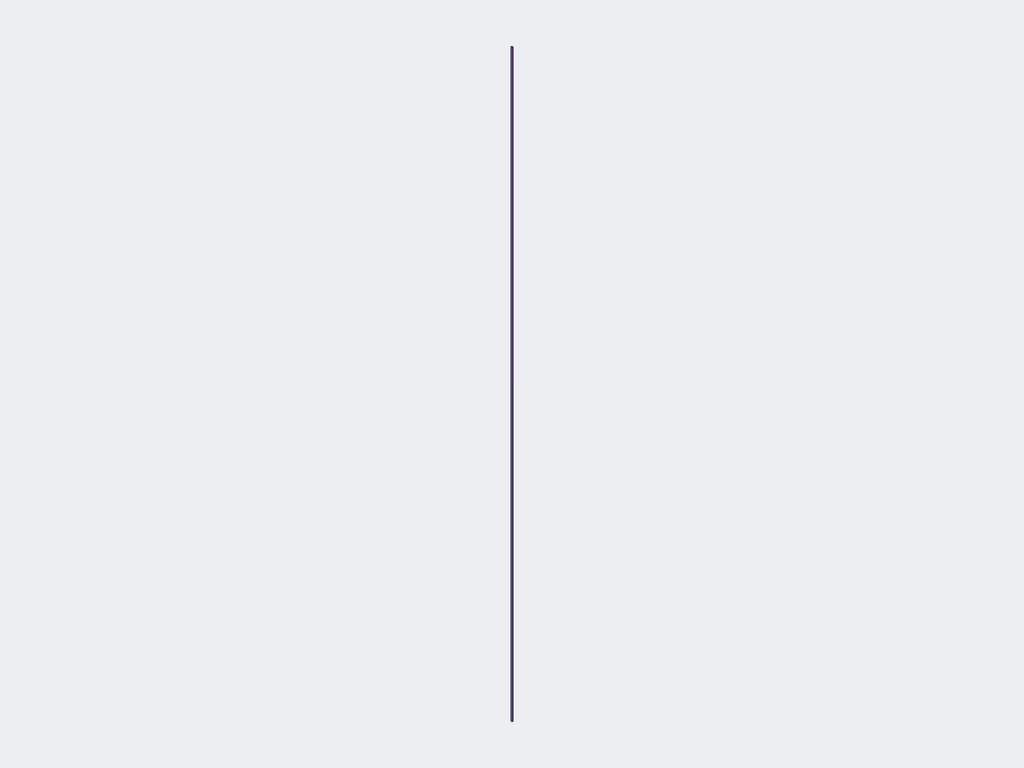Assembly | SolidWorks | 7 different items | 13 placed | box 6 x 6 x 1900 mm
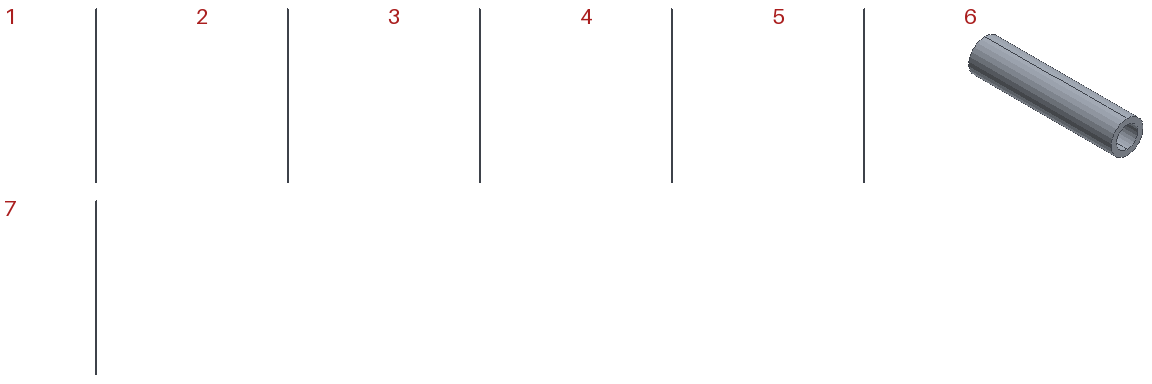Parts list (item | name | quantity | parent item | size | volume | features):
1 | (subassembly) | x1 | - | 3 x 3 x 1900 mm | 13430 mm3 | features CompositeCurve 18, Attribute 11
2 | - | x3 | in 1 | 0.15 x 0.15 x 1900 mm | 10.259 mm3 | features Extrusion 1
3 | - | x3 | in 1 | 0.3 x 0.3 x 1900 mm | 100.727 mm3 | features Extrusion 1
4 | - | x3 | in 1 | 0.125 x 0.125 x 1900 mm | 23.317 mm3 | features Extrusion 1
5 | - | x1 | in 1 | 3 x 3 x 1900 mm | 13027 mm3 | features Extrusion 1
6 | - | x1 | - | 4.5 x 20 x 4.5 mm | 176.715 mm3 | features Extrusion 1
7 | - | x1 | - | 6 x 6 x 1900 mm | 23503 mm3 | features Extrusion 1
Mates (type | each side: item.copy, entity, surface, feature):
In the top assembly
Concentric | 7.1 face cylinder Boss-Extrude1 | 6.1 face cylinder Boss-Extrude1
Coincident | 7.1 face plane Boss-Extrude1 | 6.1 face plane Boss-Extrude1
Concentric | 5.1 face cylinder Boss-Extrude1 | 6.1 face cylinder Boss-Extrude1
Coincident | 5.1 face plane Boss-Extrude1 | 7.1 face plane Boss-Extrude1
In subassembly 1
Coincident | 2.1 edge | 4.1 edge
Coincident | 3.1 edge | 2.1 edge
Coincident | 5.2 edge | 3.1 edge
Coincident | 4.2 edge | 2.2 edge
Coincident | 3.2 edge | 2.2 edge
Coincident | 5.2 edge | 3.2 edge
Coincident | 4.3 edge | 2.3 edge
Coincident | 3.3 edge | 2.3 edge
Coincident | 5.2 edge | 3.3 edge
Coincident | 2.1 face plane Boss-Extrude1 | 4.1 face plane Boss-Extrude1
Coincident | 3.1 face plane Boss-Extrude1 | 4.1 face plane Boss-Extrude1
Coincident | 4.2 face plane Boss-Extrude1 | 2.2 face plane Boss-Extrude1
Coincident | 3.2 face plane Boss-Extrude1 | 4.2 face plane Boss-Extrude1
Coincident | 4.3 face plane Boss-Extrude1 | 2.3 face plane Boss-Extrude1
Coincident | 3.3 face plane Boss-Extrude1 | 4.3 face plane Boss-Extrude1